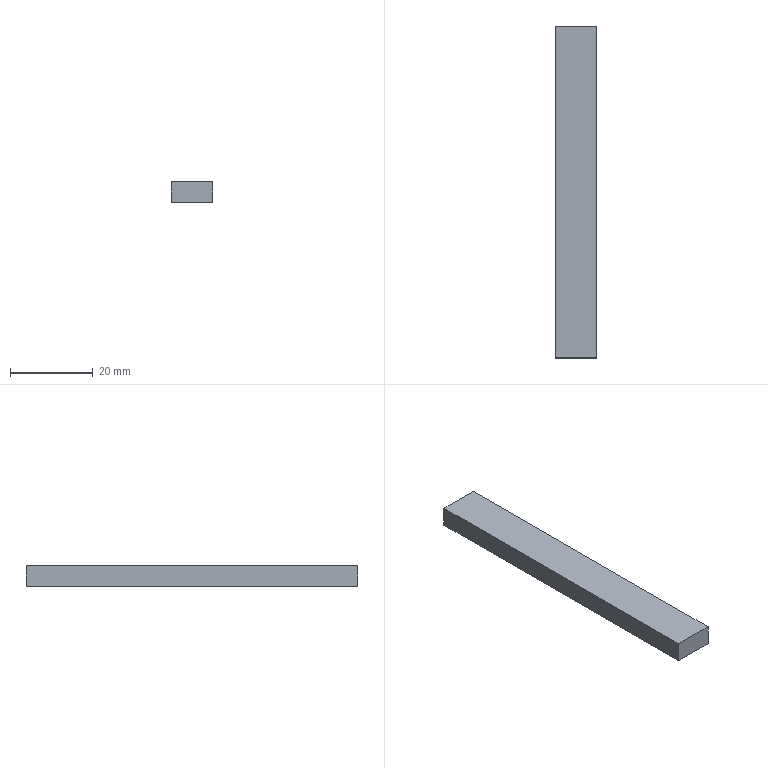Part | SolidWorks | features Extrusion 1 | 1 solid | 6 faces | box 10 x 80 x 5 mm | volume 4000 mm3 | plane 6
STEP:
#1=CARTESIAN_POINT('',(-10.,-40.,0.));
#2=VERTEX_POINT('',#1);
#3=CARTESIAN_POINT('',(0.,-40.,0.));
#4=VERTEX_POINT('',#3);
#5=CARTESIAN_POINT('',(-10.,-40.,0.));
#6=DIRECTION('',(1.,0.,0.));
#7=VECTOR('',#6,1000.);
#8=LINE('',#5,#7);
#9=EDGE_CURVE('',#2,#4,#8,.T.);
#10=ORIENTED_EDGE('',*,*,#9,.T.);
#11=CARTESIAN_POINT('',(0.,-40.,5.));
#12=VERTEX_POINT('',#11);
#13=CARTESIAN_POINT('',(0.,-40.,5.));
#14=DIRECTION('',(0.,0.,-1.));
#15=VECTOR('',#14,1000.);
#16=LINE('',#13,#15);
#17=EDGE_CURVE('',#12,#4,#16,.T.);
#18=ORIENTED_EDGE('',*,*,#17,.F.);
#19=CARTESIAN_POINT('',(-10.,-40.,5.));
#20=VERTEX_POINT('',#19);
#21=CARTESIAN_POINT('',(-10.,-40.,5.));
#22=DIRECTION('',(1.,0.,0.));
#23=VECTOR('',#22,1000.);
#24=LINE('',#21,#23);
#25=EDGE_CURVE('',#20,#12,#24,.T.);
#26=ORIENTED_EDGE('',*,*,#25,.F.);
#27=CARTESIAN_POINT('',(-10.,-40.,5.));
#28=DIRECTION('',(0.,0.,-1.));
#29=VECTOR('',#28,1000.);
#30=LINE('',#27,#29);
#31=EDGE_CURVE('',#20,#2,#30,.T.);
#32=ORIENTED_EDGE('',*,*,#31,.T.);
#33=EDGE_LOOP('',(#10,#18,#26,#32));
#34=FACE_OUTER_BOUND('',#33,.T.);
#35=CARTESIAN_POINT('',(-10.,-40.,5.));
#36=DIRECTION('',(0.,1.,0.));
#37=DIRECTION('',(0.,0.,1.));
#38=AXIS2_PLACEMENT_3D('',#35,#36,#37);
#39=PLANE('',#38);
#40=ADVANCED_FACE('',(#34),#39,.F.);
#41=CARTESIAN_POINT('',(0.,40.,0.));
#42=VERTEX_POINT('',#41);
#43=CARTESIAN_POINT('',(0.,-40.,0.));
#44=DIRECTION('',(0.,1.,0.));
#45=VECTOR('',#44,1000.);
#46=LINE('',#43,#45);
#47=EDGE_CURVE('',#4,#42,#46,.T.);
#48=ORIENTED_EDGE('',*,*,#47,.T.);
#49=CARTESIAN_POINT('',(0.,40.,5.));
#50=VERTEX_POINT('',#49);
#51=CARTESIAN_POINT('',(0.,40.,5.));
#52=DIRECTION('',(0.,0.,-1.));
#53=VECTOR('',#52,1000.);
#54=LINE('',#51,#53);
#55=EDGE_CURVE('',#50,#42,#54,.T.);
#56=ORIENTED_EDGE('',*,*,#55,.F.);
#57=CARTESIAN_POINT('',(0.,-40.,5.));
#58=DIRECTION('',(0.,1.,0.));
#59=VECTOR('',#58,1000.);
#60=LINE('',#57,#59);
#61=EDGE_CURVE('',#12,#50,#60,.T.);
#62=ORIENTED_EDGE('',*,*,#61,.F.);
#63=ORIENTED_EDGE('',*,*,#17,.T.);
#64=EDGE_LOOP('',(#48,#56,#62,#63));
#65=FACE_OUTER_BOUND('',#64,.T.);
#66=CARTESIAN_POINT('',(0.,-40.,5.));
#67=DIRECTION('',(-1.,0.,0.));
#68=DIRECTION('',(0.,0.,1.));
#69=AXIS2_PLACEMENT_3D('',#66,#67,#68);
#70=PLANE('',#69);
#71=ADVANCED_FACE('',(#65),#70,.F.);
#72=CARTESIAN_POINT('',(-10.,40.,0.));
#73=VERTEX_POINT('',#72);
#74=CARTESIAN_POINT('',(0.,40.,0.));
#75=DIRECTION('',(-1.,0.,0.));
#76=VECTOR('',#75,1000.);
#77=LINE('',#74,#76);
#78=EDGE_CURVE('',#42,#73,#77,.T.);
#79=ORIENTED_EDGE('',*,*,#78,.T.);
#80=CARTESIAN_POINT('',(-10.,40.,5.));
#81=VERTEX_POINT('',#80);
#82=CARTESIAN_POINT('',(-10.,40.,5.));
#83=DIRECTION('',(0.,0.,-1.));
#84=VECTOR('',#83,1000.);
#85=LINE('',#82,#84);
#86=EDGE_CURVE('',#81,#73,#85,.T.);
#87=ORIENTED_EDGE('',*,*,#86,.F.);
#88=CARTESIAN_POINT('',(0.,40.,5.));
#89=DIRECTION('',(-1.,0.,0.));
#90=VECTOR('',#89,1000.);
#91=LINE('',#88,#90);
#92=EDGE_CURVE('',#50,#81,#91,.T.);
#93=ORIENTED_EDGE('',*,*,#92,.F.);
#94=ORIENTED_EDGE('',*,*,#55,.T.);
#95=EDGE_LOOP('',(#79,#87,#93,#94));
#96=FACE_OUTER_BOUND('',#95,.T.);
#97=CARTESIAN_POINT('',(0.,40.,5.));
#98=DIRECTION('',(0.,-1.,0.));
#99=DIRECTION('',(1.,0.,0.));
#100=AXIS2_PLACEMENT_3D('',#97,#98,#99);
#101=PLANE('',#100);
#102=ADVANCED_FACE('',(#96),#101,.F.);
#103=CARTESIAN_POINT('',(-10.,40.,0.));
#104=DIRECTION('',(0.,-1.,0.));
#105=VECTOR('',#104,1000.);
#106=LINE('',#103,#105);
#107=EDGE_CURVE('',#73,#2,#106,.T.);
#108=ORIENTED_EDGE('',*,*,#107,.T.);
#109=ORIENTED_EDGE('',*,*,#31,.F.);
#110=CARTESIAN_POINT('',(-10.,40.,5.));
#111=DIRECTION('',(0.,-1.,0.));
#112=VECTOR('',#111,1000.);
#113=LINE('',#110,#112);
#114=EDGE_CURVE('',#81,#20,#113,.T.);
#115=ORIENTED_EDGE('',*,*,#114,.F.);
#116=ORIENTED_EDGE('',*,*,#86,.T.);
#117=EDGE_LOOP('',(#108,#109,#115,#116));
#118=FACE_OUTER_BOUND('',#117,.T.);
#119=CARTESIAN_POINT('',(-10.,40.,5.));
#120=DIRECTION('',(1.,0.,0.));
#121=DIRECTION('',(0.,0.,-1.));
#122=AXIS2_PLACEMENT_3D('',#119,#120,#121);
#123=PLANE('',#122);
#124=ADVANCED_FACE('',(#118),#123,.F.);
#125=ORIENTED_EDGE('',*,*,#25,.T.);
#126=ORIENTED_EDGE('',*,*,#61,.T.);
#127=ORIENTED_EDGE('',*,*,#92,.T.);
#128=ORIENTED_EDGE('',*,*,#114,.T.);
#129=EDGE_LOOP('',(#125,#126,#127,#128));
#130=FACE_OUTER_BOUND('',#129,.T.);
#131=CARTESIAN_POINT('',(0.,-40.,5.));
#132=DIRECTION('',(0.,0.,1.));
#133=DIRECTION('',(1.,0.,0.));
#134=AXIS2_PLACEMENT_3D('',#131,#132,#133);
#135=PLANE('',#134);
#136=ADVANCED_FACE('',(#130),#135,.T.);
#137=ORIENTED_EDGE('',*,*,#9,.F.);
#138=ORIENTED_EDGE('',*,*,#107,.F.);
#139=ORIENTED_EDGE('',*,*,#78,.F.);
#140=ORIENTED_EDGE('',*,*,#47,.F.);
#141=EDGE_LOOP('',(#137,#138,#139,#140));
#142=FACE_OUTER_BOUND('',#141,.T.);
#143=CARTESIAN_POINT('',(0.,-40.,0.));
#144=DIRECTION('',(0.,0.,1.));
#145=DIRECTION('',(1.,0.,0.));
#146=AXIS2_PLACEMENT_3D('',#143,#144,#145);
#147=PLANE('',#146);
#148=ADVANCED_FACE('',(#142),#147,.F.);
#149=CLOSED_SHELL('',(#40,#71,#102,#124,#136,#148));
#150=MANIFOLD_SOLID_BREP('',#149);
#151=CARTESIAN_POINT('',(0.,0.,0.));
#152=DIRECTION('',(0.,0.,1.));
#153=DIRECTION('',(1.,0.,0.));
#154=AXIS2_PLACEMENT_3D('',#151,#152,#153);
#155=(LENGTH_UNIT()NAMED_UNIT(*)SI_UNIT(.MILLI.,.METRE.));
#156=UNCERTAINTY_MEASURE_WITH_UNIT(LENGTH_MEASURE(0.00001),#155,'','');
#157=(NAMED_UNIT(*)PLANE_ANGLE_UNIT()SI_UNIT($,.RADIAN.));
#158=(NAMED_UNIT(*)SI_UNIT($,.STERADIAN.)SOLID_ANGLE_UNIT());
#159=(GEOMETRIC_REPRESENTATION_CONTEXT(3)GLOBAL_UNCERTAINTY_ASSIGNED_CONTEXT((#156))GLOBAL_UNIT_ASSIGNED_CONTEXT((#155,#157,#158))REPRESENTATION_CONTEXT('',''));
#160=ADVANCED_BREP_SHAPE_REPRESENTATION('',(#150,#154),#159);